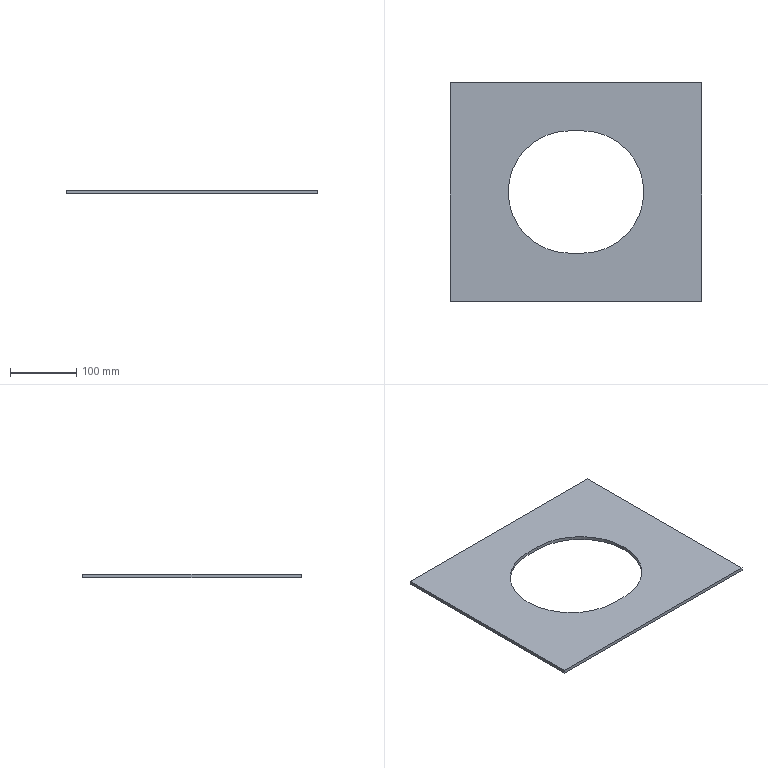Part | SolidWorks | features Cut 1, Extrusion 1, ICE 1 | 1 solid | 11 faces | box 380 x 330 x 5 mm | volume 474099 mm3 | plane 8 | cylinder 3 | commonest cylinder face diameters 185 x3
STEP:
#1=CARTESIAN_POINT('',(87.5,165.,5.));
#2=VERTEX_POINT('',#1);
#3=CARTESIAN_POINT('',(180.,257.5,5.));
#4=VERTEX_POINT('',#3);
#5=CARTESIAN_POINT('',(180.,165.,5.));
#6=DIRECTION('',(0.,0.,-1.));
#7=DIRECTION('',(-1.,0.,0.));
#8=AXIS2_PLACEMENT_3D('',#5,#6,#7);
#9=CIRCLE('',#8,92.5);
#10=EDGE_CURVE('',#2,#4,#9,.T.);
#11=ORIENTED_EDGE('',*,*,#10,.F.);
#12=CARTESIAN_POINT('',(87.5,165.,0.));
#13=VERTEX_POINT('',#12);
#14=CARTESIAN_POINT('',(87.5,165.,5.));
#15=DIRECTION('',(0.,0.,-1.));
#16=VECTOR('',#15,1000.);
#17=LINE('',#14,#16);
#18=EDGE_CURVE('',#2,#13,#17,.T.);
#19=ORIENTED_EDGE('',*,*,#18,.T.);
#20=CARTESIAN_POINT('',(180.,257.5,0.));
#21=VERTEX_POINT('',#20);
#22=CARTESIAN_POINT('',(180.,165.,0.));
#23=DIRECTION('',(0.,0.,-1.));
#24=DIRECTION('',(-1.,0.,0.));
#25=AXIS2_PLACEMENT_3D('',#22,#23,#24);
#26=CIRCLE('',#25,92.5);
#27=EDGE_CURVE('',#13,#21,#26,.T.);
#28=ORIENTED_EDGE('',*,*,#27,.T.);
#29=CARTESIAN_POINT('',(180.,257.5,5.));
#30=DIRECTION('',(0.,0.,-1.));
#31=VECTOR('',#30,1000.);
#32=LINE('',#29,#31);
#33=EDGE_CURVE('',#4,#21,#32,.T.);
#34=ORIENTED_EDGE('',*,*,#33,.F.);
#35=EDGE_LOOP('',(#11,#19,#28,#34));
#36=FACE_OUTER_BOUND('',#35,.T.);
#37=CARTESIAN_POINT('',(180.,165.,5.));
#38=DIRECTION('',(0.,0.,-1.));
#39=DIRECTION('',(-1.,0.,0.));
#40=AXIS2_PLACEMENT_3D('',#37,#38,#39);
#41=CYLINDRICAL_SURFACE('',#40,92.5);
#42=ADVANCED_FACE('',(#36),#41,.F.);
#43=CARTESIAN_POINT('',(180.,72.5,5.));
#44=VERTEX_POINT('',#43);
#45=CARTESIAN_POINT('',(180.,72.5,0.));
#46=VERTEX_POINT('',#45);
#47=CARTESIAN_POINT('',(180.,72.5,5.));
#48=DIRECTION('',(0.,0.,-1.));
#49=VECTOR('',#48,1000.);
#50=LINE('',#47,#49);
#51=EDGE_CURVE('',#44,#46,#50,.T.);
#52=ORIENTED_EDGE('',*,*,#51,.F.);
#53=CARTESIAN_POINT('',(200.,72.5,5.));
#54=VERTEX_POINT('',#53);
#55=CARTESIAN_POINT('',(0.,72.5,5.));
#56=DIRECTION('',(1.,0.,0.));
#57=VECTOR('',#56,1000.);
#58=LINE('',#55,#57);
#59=EDGE_CURVE('',#44,#54,#58,.T.);
#60=ORIENTED_EDGE('',*,*,#59,.T.);
#61=CARTESIAN_POINT('',(200.,72.5,0.));
#62=VERTEX_POINT('',#61);
#63=CARTESIAN_POINT('',(200.,72.5,5.));
#64=DIRECTION('',(0.,0.,-1.));
#65=VECTOR('',#64,1000.);
#66=LINE('',#63,#65);
#67=EDGE_CURVE('',#54,#62,#66,.T.);
#68=ORIENTED_EDGE('',*,*,#67,.T.);
#69=CARTESIAN_POINT('',(0.,72.5,0.));
#70=DIRECTION('',(-1.,0.,0.));
#71=VECTOR('',#70,1000.);
#72=LINE('',#69,#71);
#73=EDGE_CURVE('',#62,#46,#72,.T.);
#74=ORIENTED_EDGE('',*,*,#73,.T.);
#75=EDGE_LOOP('',(#52,#60,#68,#74));
#76=FACE_OUTER_BOUND('',#75,.T.);
#77=CARTESIAN_POINT('',(0.,72.5,10.));
#78=DIRECTION('',(0.,-1.,0.));
#79=DIRECTION('',(0.,0.,-1.));
#80=AXIS2_PLACEMENT_3D('',#77,#78,#79);
#81=PLANE('',#80);
#82=ADVANCED_FACE('',(#76),#81,.F.);
#83=CARTESIAN_POINT('',(200.,257.5,5.));
#84=VERTEX_POINT('',#83);
#85=CARTESIAN_POINT('',(0.,257.5,5.));
#86=DIRECTION('',(1.,0.,0.));
#87=VECTOR('',#86,1000.);
#88=LINE('',#85,#87);
#89=EDGE_CURVE('',#4,#84,#88,.T.);
#90=ORIENTED_EDGE('',*,*,#89,.F.);
#91=ORIENTED_EDGE('',*,*,#33,.T.);
#92=CARTESIAN_POINT('',(200.,257.5,0.));
#93=VERTEX_POINT('',#92);
#94=CARTESIAN_POINT('',(0.,257.5,0.));
#95=DIRECTION('',(-1.,0.,0.));
#96=VECTOR('',#95,1000.);
#97=LINE('',#94,#96);
#98=EDGE_CURVE('',#93,#21,#97,.T.);
#99=ORIENTED_EDGE('',*,*,#98,.F.);
#100=CARTESIAN_POINT('',(200.,257.5,5.));
#101=DIRECTION('',(0.,0.,-1.));
#102=VECTOR('',#101,1000.);
#103=LINE('',#100,#102);
#104=EDGE_CURVE('',#84,#93,#103,.T.);
#105=ORIENTED_EDGE('',*,*,#104,.F.);
#106=EDGE_LOOP('',(#90,#91,#99,#105));
#107=FACE_OUTER_BOUND('',#106,.T.);
#108=CARTESIAN_POINT('',(0.,257.5,10.));
#109=DIRECTION('',(0.,-1.,0.));
#110=DIRECTION('',(0.,0.,-1.));
#111=AXIS2_PLACEMENT_3D('',#108,#109,#110);
#112=PLANE('',#111);
#113=ADVANCED_FACE('',(#107),#112,.T.);
#114=CARTESIAN_POINT('',(0.,330.,0.));
#115=VERTEX_POINT('',#114);
#116=CARTESIAN_POINT('',(0.,0.,0.));
#117=VERTEX_POINT('',#116);
#118=CARTESIAN_POINT('',(0.,330.,0.));
#119=DIRECTION('',(0.,-1.,0.));
#120=VECTOR('',#119,1000.);
#121=LINE('',#118,#120);
#122=EDGE_CURVE('',#115,#117,#121,.T.);
#123=ORIENTED_EDGE('',*,*,#122,.T.);
#124=CARTESIAN_POINT('',(0.,0.,5.));
#125=VERTEX_POINT('',#124);
#126=CARTESIAN_POINT('',(0.,0.,5.));
#127=DIRECTION('',(0.,0.,-1.));
#128=VECTOR('',#127,1000.);
#129=LINE('',#126,#128);
#130=EDGE_CURVE('',#125,#117,#129,.T.);
#131=ORIENTED_EDGE('',*,*,#130,.F.);
#132=CARTESIAN_POINT('',(0.,330.,5.));
#133=VERTEX_POINT('',#132);
#134=CARTESIAN_POINT('',(0.,330.,5.));
#135=DIRECTION('',(0.,-1.,0.));
#136=VECTOR('',#135,1000.);
#137=LINE('',#134,#136);
#138=EDGE_CURVE('',#133,#125,#137,.T.);
#139=ORIENTED_EDGE('',*,*,#138,.F.);
#140=CARTESIAN_POINT('',(0.,330.,5.));
#141=DIRECTION('',(0.,0.,-1.));
#142=VECTOR('',#141,1000.);
#143=LINE('',#140,#142);
#144=EDGE_CURVE('',#133,#115,#143,.T.);
#145=ORIENTED_EDGE('',*,*,#144,.T.);
#146=EDGE_LOOP('',(#123,#131,#139,#145));
#147=FACE_OUTER_BOUND('',#146,.T.);
#148=CARTESIAN_POINT('',(0.,330.,5.));
#149=DIRECTION('',(1.,0.,0.));
#150=DIRECTION('',(0.,0.,-1.));
#151=AXIS2_PLACEMENT_3D('',#148,#149,#150);
#152=PLANE('',#151);
#153=ADVANCED_FACE('',(#147),#152,.F.);
#154=CARTESIAN_POINT('',(380.,0.,0.));
#155=VERTEX_POINT('',#154);
#156=CARTESIAN_POINT('',(0.,0.,0.));
#157=DIRECTION('',(1.,0.,0.));
#158=VECTOR('',#157,1000.);
#159=LINE('',#156,#158);
#160=EDGE_CURVE('',#117,#155,#159,.T.);
#161=ORIENTED_EDGE('',*,*,#160,.T.);
#162=CARTESIAN_POINT('',(380.,0.,5.));
#163=VERTEX_POINT('',#162);
#164=CARTESIAN_POINT('',(380.,0.,5.));
#165=DIRECTION('',(0.,0.,-1.));
#166=VECTOR('',#165,1000.);
#167=LINE('',#164,#166);
#168=EDGE_CURVE('',#163,#155,#167,.T.);
#169=ORIENTED_EDGE('',*,*,#168,.F.);
#170=CARTESIAN_POINT('',(0.,0.,5.));
#171=DIRECTION('',(1.,0.,0.));
#172=VECTOR('',#171,1000.);
#173=LINE('',#170,#172);
#174=EDGE_CURVE('',#125,#163,#173,.T.);
#175=ORIENTED_EDGE('',*,*,#174,.F.);
#176=ORIENTED_EDGE('',*,*,#130,.T.);
#177=EDGE_LOOP('',(#161,#169,#175,#176));
#178=FACE_OUTER_BOUND('',#177,.T.);
#179=CARTESIAN_POINT('',(0.,0.,5.));
#180=DIRECTION('',(0.,1.,0.));
#181=DIRECTION('',(0.,0.,1.));
#182=AXIS2_PLACEMENT_3D('',#179,#180,#181);
#183=PLANE('',#182);
#184=ADVANCED_FACE('',(#178),#183,.F.);
#185=CARTESIAN_POINT('',(380.,330.,0.));
#186=VERTEX_POINT('',#185);
#187=CARTESIAN_POINT('',(380.,0.,0.));
#188=DIRECTION('',(0.,1.,0.));
#189=VECTOR('',#188,1000.);
#190=LINE('',#187,#189);
#191=EDGE_CURVE('',#155,#186,#190,.T.);
#192=ORIENTED_EDGE('',*,*,#191,.T.);
#193=CARTESIAN_POINT('',(380.,330.,5.));
#194=VERTEX_POINT('',#193);
#195=CARTESIAN_POINT('',(380.,330.,5.));
#196=DIRECTION('',(0.,0.,-1.));
#197=VECTOR('',#196,1000.);
#198=LINE('',#195,#197);
#199=EDGE_CURVE('',#194,#186,#198,.T.);
#200=ORIENTED_EDGE('',*,*,#199,.F.);
#201=CARTESIAN_POINT('',(380.,0.,5.));
#202=DIRECTION('',(0.,1.,0.));
#203=VECTOR('',#202,1000.);
#204=LINE('',#201,#203);
#205=EDGE_CURVE('',#163,#194,#204,.T.);
#206=ORIENTED_EDGE('',*,*,#205,.F.);
#207=ORIENTED_EDGE('',*,*,#168,.T.);
#208=EDGE_LOOP('',(#192,#200,#206,#207));
#209=FACE_OUTER_BOUND('',#208,.T.);
#210=CARTESIAN_POINT('',(380.,0.,5.));
#211=DIRECTION('',(-1.,0.,0.));
#212=DIRECTION('',(0.,0.,1.));
#213=AXIS2_PLACEMENT_3D('',#210,#211,#212);
#214=PLANE('',#213);
#215=ADVANCED_FACE('',(#209),#214,.F.);
#216=CARTESIAN_POINT('',(380.,330.,0.));
#217=DIRECTION('',(-1.,0.,0.));
#218=VECTOR('',#217,1000.);
#219=LINE('',#216,#218);
#220=EDGE_CURVE('',#186,#115,#219,.T.);
#221=ORIENTED_EDGE('',*,*,#220,.T.);
#222=ORIENTED_EDGE('',*,*,#144,.F.);
#223=CARTESIAN_POINT('',(380.,330.,5.));
#224=DIRECTION('',(-1.,0.,0.));
#225=VECTOR('',#224,1000.);
#226=LINE('',#223,#225);
#227=EDGE_CURVE('',#194,#133,#226,.T.);
#228=ORIENTED_EDGE('',*,*,#227,.F.);
#229=ORIENTED_EDGE('',*,*,#199,.T.);
#230=EDGE_LOOP('',(#221,#222,#228,#229));
#231=FACE_OUTER_BOUND('',#230,.T.);
#232=CARTESIAN_POINT('',(380.,330.,5.));
#233=DIRECTION('',(0.,-1.,0.));
#234=DIRECTION('',(0.,0.,-1.));
#235=AXIS2_PLACEMENT_3D('',#232,#233,#234);
#236=PLANE('',#235);
#237=ADVANCED_FACE('',(#231),#236,.F.);
#238=ORIENTED_EDGE('',*,*,#59,.F.);
#239=CARTESIAN_POINT('',(180.,165.,5.));
#240=DIRECTION('',(0.,0.,-1.));
#241=DIRECTION('',(-1.,0.,0.));
#242=AXIS2_PLACEMENT_3D('',#239,#240,#241);
#243=CIRCLE('',#242,92.5);
#244=EDGE_CURVE('',#44,#2,#243,.T.);
#245=ORIENTED_EDGE('',*,*,#244,.T.);
#246=ORIENTED_EDGE('',*,*,#10,.T.);
#247=ORIENTED_EDGE('',*,*,#89,.T.);
#248=CARTESIAN_POINT('',(200.,165.,5.));
#249=DIRECTION('',(0.,0.,-1.));
#250=DIRECTION('',(-1.,0.,0.));
#251=AXIS2_PLACEMENT_3D('',#248,#249,#250);
#252=CIRCLE('',#251,92.5);
#253=EDGE_CURVE('',#84,#54,#252,.T.);
#254=ORIENTED_EDGE('',*,*,#253,.T.);
#255=EDGE_LOOP('',(#238,#245,#246,#247,#254));
#256=FACE_BOUND('',#255,.T.);
#257=ORIENTED_EDGE('',*,*,#138,.T.);
#258=ORIENTED_EDGE('',*,*,#174,.T.);
#259=ORIENTED_EDGE('',*,*,#205,.T.);
#260=ORIENTED_EDGE('',*,*,#227,.T.);
#261=EDGE_LOOP('',(#257,#258,#259,#260));
#262=FACE_OUTER_BOUND('',#261,.T.);
#263=CARTESIAN_POINT('',(0.,0.,5.));
#264=DIRECTION('',(0.,0.,1.));
#265=DIRECTION('',(1.,0.,0.));
#266=AXIS2_PLACEMENT_3D('',#263,#264,#265);
#267=PLANE('',#266);
#268=ADVANCED_FACE('',(#256,#262),#267,.T.);
#269=CARTESIAN_POINT('',(180.,165.,0.));
#270=DIRECTION('',(0.,0.,-1.));
#271=DIRECTION('',(-1.,0.,0.));
#272=AXIS2_PLACEMENT_3D('',#269,#270,#271);
#273=CIRCLE('',#272,92.5);
#274=EDGE_CURVE('',#46,#13,#273,.T.);
#275=ORIENTED_EDGE('',*,*,#274,.F.);
#276=ORIENTED_EDGE('',*,*,#73,.F.);
#277=CARTESIAN_POINT('',(200.,165.,0.));
#278=DIRECTION('',(0.,0.,-1.));
#279=DIRECTION('',(-1.,0.,0.));
#280=AXIS2_PLACEMENT_3D('',#277,#278,#279);
#281=CIRCLE('',#280,92.5);
#282=EDGE_CURVE('',#93,#62,#281,.T.);
#283=ORIENTED_EDGE('',*,*,#282,.F.);
#284=ORIENTED_EDGE('',*,*,#98,.T.);
#285=ORIENTED_EDGE('',*,*,#27,.F.);
#286=EDGE_LOOP('',(#275,#276,#283,#284,#285));
#287=FACE_BOUND('',#286,.T.);
#288=ORIENTED_EDGE('',*,*,#122,.F.);
#289=ORIENTED_EDGE('',*,*,#220,.F.);
#290=ORIENTED_EDGE('',*,*,#191,.F.);
#291=ORIENTED_EDGE('',*,*,#160,.F.);
#292=EDGE_LOOP('',(#288,#289,#290,#291));
#293=FACE_OUTER_BOUND('',#292,.T.);
#294=CARTESIAN_POINT('',(0.,0.,0.));
#295=DIRECTION('',(0.,0.,1.));
#296=DIRECTION('',(1.,0.,0.));
#297=AXIS2_PLACEMENT_3D('',#294,#295,#296);
#298=PLANE('',#297);
#299=ADVANCED_FACE('',(#287,#293),#298,.F.);
#300=ORIENTED_EDGE('',*,*,#282,.T.);
#301=ORIENTED_EDGE('',*,*,#67,.F.);
#302=ORIENTED_EDGE('',*,*,#253,.F.);
#303=ORIENTED_EDGE('',*,*,#104,.T.);
#304=EDGE_LOOP('',(#300,#301,#302,#303));
#305=FACE_OUTER_BOUND('',#304,.T.);
#306=CARTESIAN_POINT('',(200.,165.,5.));
#307=DIRECTION('',(0.,0.,-1.));
#308=DIRECTION('',(-1.,0.,0.));
#309=AXIS2_PLACEMENT_3D('',#306,#307,#308);
#310=CYLINDRICAL_SURFACE('',#309,92.5);
#311=ADVANCED_FACE('',(#305),#310,.F.);
#312=ORIENTED_EDGE('',*,*,#18,.F.);
#313=ORIENTED_EDGE('',*,*,#244,.F.);
#314=ORIENTED_EDGE('',*,*,#51,.T.);
#315=ORIENTED_EDGE('',*,*,#274,.T.);
#316=EDGE_LOOP('',(#312,#313,#314,#315));
#317=FACE_OUTER_BOUND('',#316,.T.);
#318=CARTESIAN_POINT('',(180.,165.,5.));
#319=DIRECTION('',(0.,0.,-1.));
#320=DIRECTION('',(-1.,0.,0.));
#321=AXIS2_PLACEMENT_3D('',#318,#319,#320);
#322=CYLINDRICAL_SURFACE('',#321,92.5);
#323=ADVANCED_FACE('',(#317),#322,.F.);
#324=CLOSED_SHELL('',(#42,#82,#113,#153,#184,#215,#237,#268,#299,#311,#323));
#325=MANIFOLD_SOLID_BREP('',#324);
#326=CARTESIAN_POINT('',(0.,0.,0.));
#327=DIRECTION('',(0.,0.,1.));
#328=DIRECTION('',(1.,0.,0.));
#329=AXIS2_PLACEMENT_3D('',#326,#327,#328);
#330=(LENGTH_UNIT()NAMED_UNIT(*)SI_UNIT(.MILLI.,.METRE.));
#331=UNCERTAINTY_MEASURE_WITH_UNIT(LENGTH_MEASURE(0.00001),#330,'','');
#332=(NAMED_UNIT(*)PLANE_ANGLE_UNIT()SI_UNIT($,.RADIAN.));
#333=(NAMED_UNIT(*)SI_UNIT($,.STERADIAN.)SOLID_ANGLE_UNIT());
#334=(GEOMETRIC_REPRESENTATION_CONTEXT(3)GLOBAL_UNCERTAINTY_ASSIGNED_CONTEXT((#331))GLOBAL_UNIT_ASSIGNED_CONTEXT((#330,#332,#333))REPRESENTATION_CONTEXT('',''));
#335=ADVANCED_BREP_SHAPE_REPRESENTATION('',(#325,#329),#334);